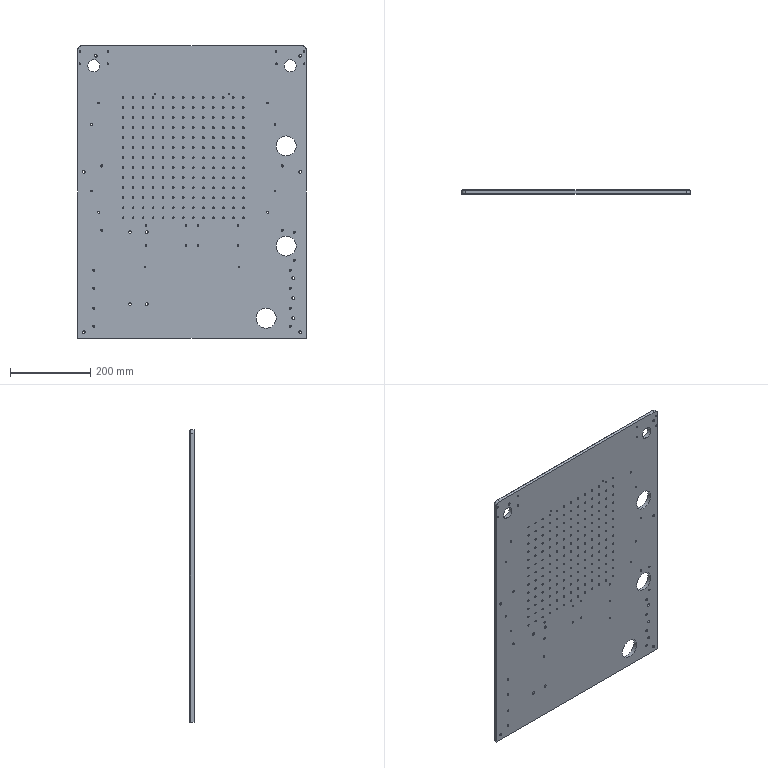Part | SolidWorks | features HoleWzd 11, Cut 2, Chamfer 1, Extrusion 1, Fillet 1, ICE 1, LPattern 1 | 1 solid | 490 faces | box 570 x 10 x 730 mm | volume 4046206 mm3 | cylinder 473 | plane 15 | cone 2 | commonest cylinder face diameters 4.2 x395 5.2 x24 6.6 x12 11 x12 6.8 x8 7 x6